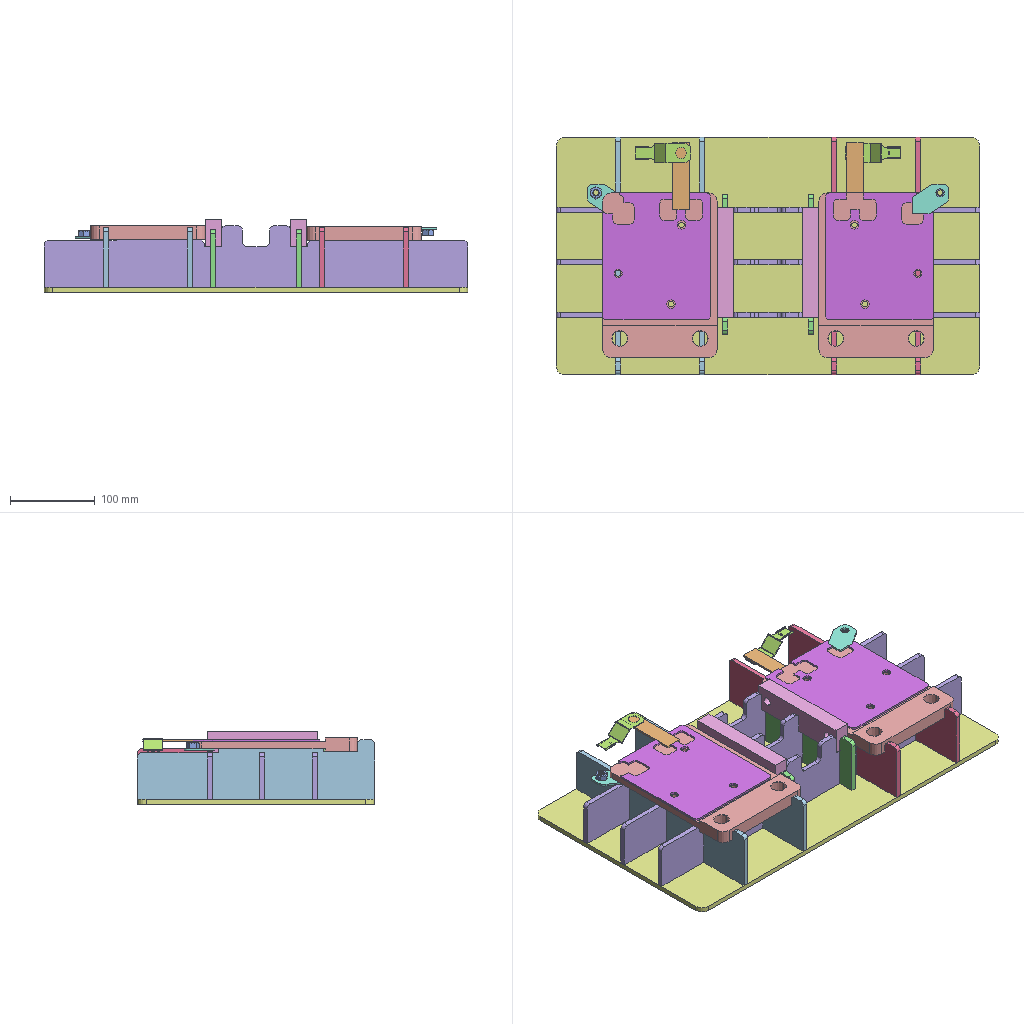Assembly | SolidWorks | 13 different items | 26 placed | box 500 x 280 x 86 mm
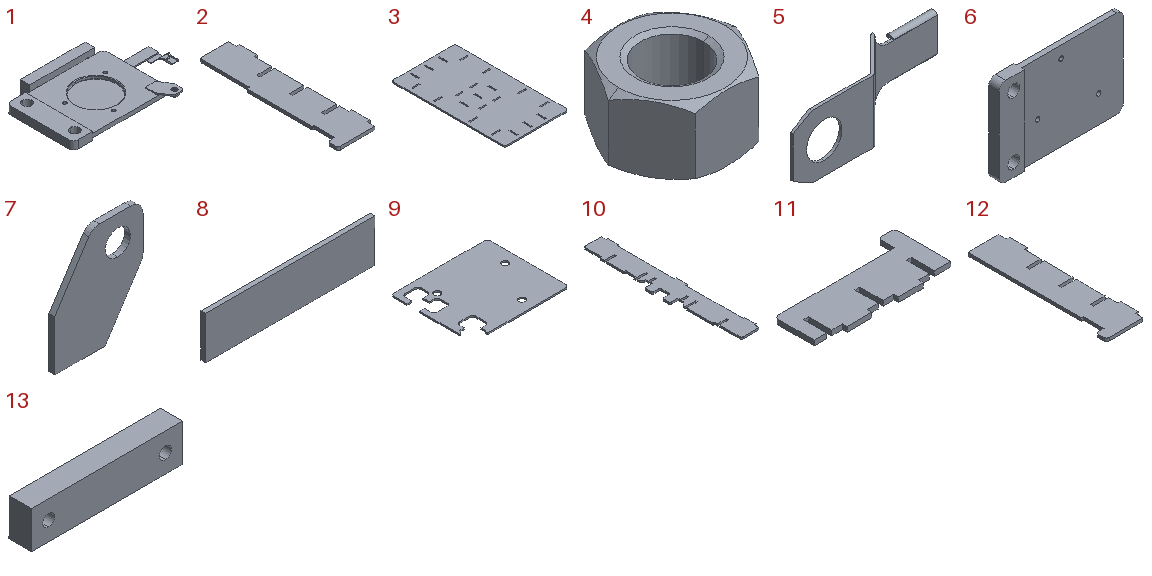Parts list (item | name | quantity | parent item | size | volume | features):
1 | (subassembly) | x2 | - | 253.5 x 172 x 32 mm | 295798 mm3 | -
2 | - | x2 | - | 76 x 280 x 6 mm | 97544 mm3 | features Fillet 1, FlatPattern 1, SMBaseFlange 1, SheetMetal 1
3 | - | x1 | - | 280 x 500 x 6 mm | 813715 mm3 | features FlatPattern 1, SMBaseFlange 1, SheetMetal 1
4 | - | x2 | in 1 | 27.713 x 24 x 14.8 mm | 5071 mm3 | features RevCut 2, Chamfer 1, Extrusion 1, LPattern 1
5 | - | x2 | in 1 | 65.7 x 15.573 x 23.06 mm | 1342 mm3 | features BaseBody 1
6 | - | x2 | in 1 | 194.5 x 16 x 135 mm | 211709 mm3 | features ICE 4, Chamfer 2, Fillet 1, FlatPattern 1, HoleWzd 1, SMBaseFlange 1, SheetMetal 1
7 | - | x2 | in 1 | 35 x 2.3 x 43 mm | 2472 mm3 | features FlatPattern 1, SMBaseFlange 1, SheetMetal 1
8 | - | x2 | in 1 | 79 x 2.3 x 20 mm | 3634 mm3 | features FlatPattern 1, SMBaseFlange 1, SheetMetal 1
9 | - | x2 | - | 150 x 127 x 2.3 mm | 37985 mm3 | features Fillet 1, FlatPattern 1, SMBaseFlange 1, SheetMetal 1
10 | - | x3 | - | 78 x 500 x 6 mm | 170412 mm3 | features Fillet 1, FlatPattern 1, SMBaseFlange 1, SheetMetal 1
11 | - | x2 | - | 165 x 73.5 x 6 mm | 48779 mm3 | features Fillet 1, FlatPattern 1, SMBaseFlange 1, SheetMetal 1
12 | - | x2 | - | 76 x 280 x 6 mm | 100169 mm3 | features Fillet 1, FlatPattern 1, SMBaseFlange 1, SheetMetal 1
13 | - | x2 | in 1 | 130 x 19 x 32 mm | 75935 mm3 | features FlatPattern 1, HoleWzd 1, SMBaseFlange 1, SheetMetal 1
Mates (type | each side: item.copy, entity, surface, feature):
In the top assembly
Coincident | 1.1 face | 11.1 face plane Base-Flange1 | 2 times
DistanceDim | 1.1 face | 11.1 face plane Base-Flange1
InPlace | 10.1 face plane Base-Flange1 | 3.1 plane
Coincident | 1.1 face | 9.1 face plane Base-Flange1
Concentric | 1.1 face | 9.1 face cylinder Base-Flange1 | 2 times
In subassembly 1
Parallel | 6.1 face plane Base-Flange1 | 5.1 face plane Input 1
Coincident | 6.1 face plane Base-Flange1 | 13.1 face plane Base-Flange1
DistanceDim | 13.1 face plane Base-Flange1 | 6.1 face plane Base-Flange1
DistanceDim | 6.1 face plane Cut-Extrude1 | 13.1 face plane Base-Flange1
Coincident | 6.1 face plane Cut-Extrude1 | 7.1 face plane Base-Flange1
DistanceDim | 6.1 face plane Base-Flange1 | 7.1 face plane Base-Flange1
DistanceDim | 7.1 face plane Base-Flange1 | 6.1 face plane Base-Flange1
Coincident | 4.1 face plane BaseNut | 7.1 face plane Base-Flange1
Concentric | 4.1 face cone LPattern10 | 7.1 face cylinder Base-Flange1
Parallel | 4.1 face plane BaseNut | 7.1 face plane Base-Flange1
Coincident | 6.1 face plane Cut-Extrude2 | 8.1 face plane Base-Flange1
DistanceDim | 6.1 face plane Base-Flange1 | 8.1 face plane Base-Flange1 | 2 times
Coincident | 5.1 face plane Input 1 | 8.1 face plane Base-Flange1
DistanceDim | 5.1 face cylinder Input 1 | 8.1 face plane Base-Flange1
DistanceDim | 5.1 face cylinder Input 1 | 6.1 face plane Base-Flange1